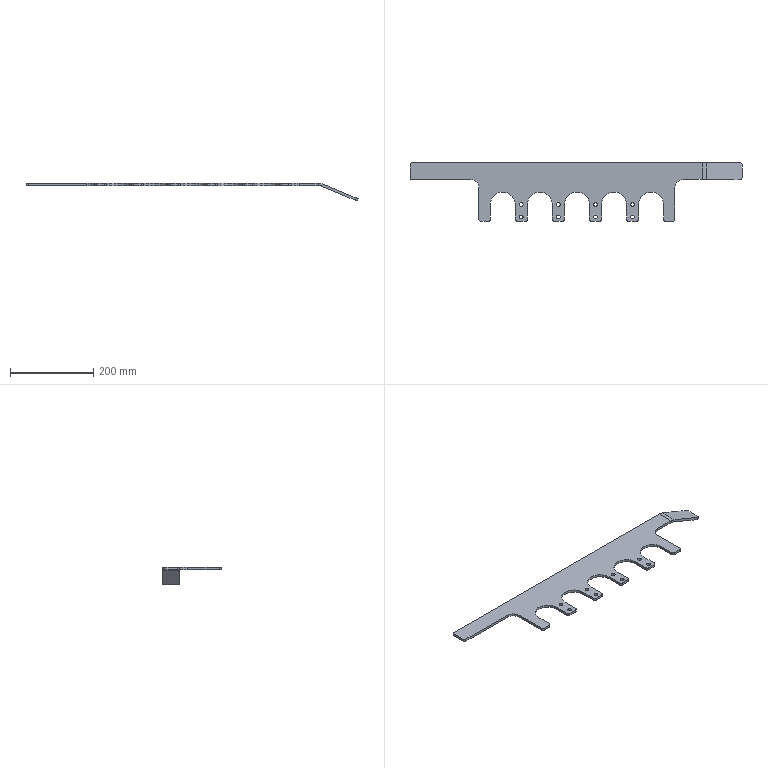Part | SolidWorks | features BaseBody 1 | 1 solid | 72 faces | box 795.553 x 140 x 42.981 mm | volume 357455 mm3 | cylinder 41 | plane 31 | commonest cylinder face diameters 9 x16 10 x16 60 x5 40 x3 52 x1